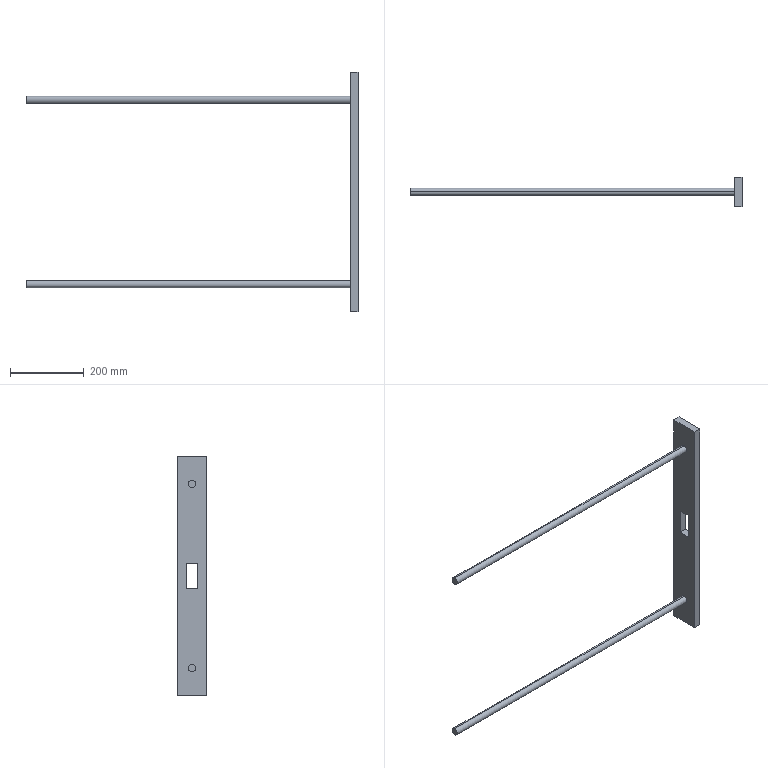Part | SolidWorks | features ICE 2, Extrusion 1 | 1 solid | 16 faces | box 900 x 80 x 650 mm | volume 1550920 mm3 | plane 12 | cylinder 4 | commonest cylinder face diameters 20 x4
STEP:
#1=CARTESIAN_POINT('',(-880.,0.,240.));
#2=VERTEX_POINT('',#1);
#3=CARTESIAN_POINT('',(-880.,0.,260.));
#4=VERTEX_POINT('',#3);
#5=CARTESIAN_POINT('',(-880.,0.,250.));
#6=DIRECTION('',(1.,0.,0.));
#7=DIRECTION('',(0.,0.,-1.));
#8=AXIS2_PLACEMENT_3D('',#5,#6,#7);
#9=CIRCLE('',#8,10.);
#10=EDGE_CURVE('',#2,#4,#9,.T.);
#11=ORIENTED_EDGE('',*,*,#10,.T.);
#12=CARTESIAN_POINT('',(0.,0.,260.));
#13=VERTEX_POINT('',#12);
#14=CARTESIAN_POINT('',(-880.,0.,260.));
#15=DIRECTION('',(1.,0.,0.));
#16=VECTOR('',#15,1000.);
#17=LINE('',#14,#16);
#18=EDGE_CURVE('',#4,#13,#17,.T.);
#19=ORIENTED_EDGE('',*,*,#18,.T.);
#20=CARTESIAN_POINT('',(0.,0.,240.));
#21=VERTEX_POINT('',#20);
#22=CARTESIAN_POINT('',(0.,0.,250.));
#23=DIRECTION('',(1.,0.,0.));
#24=DIRECTION('',(0.,0.,-1.));
#25=AXIS2_PLACEMENT_3D('',#22,#23,#24);
#26=CIRCLE('',#25,10.);
#27=EDGE_CURVE('',#21,#13,#26,.T.);
#28=ORIENTED_EDGE('',*,*,#27,.F.);
#29=CARTESIAN_POINT('',(-880.,0.,240.));
#30=DIRECTION('',(1.,0.,0.));
#31=VECTOR('',#30,1000.);
#32=LINE('',#29,#31);
#33=EDGE_CURVE('',#2,#21,#32,.T.);
#34=ORIENTED_EDGE('',*,*,#33,.F.);
#35=EDGE_LOOP('',(#11,#19,#28,#34));
#36=FACE_OUTER_BOUND('',#35,.T.);
#37=CARTESIAN_POINT('',(-880.,0.,250.));
#38=DIRECTION('',(1.,0.,0.));
#39=DIRECTION('',(0.,0.,-1.));
#40=AXIS2_PLACEMENT_3D('',#37,#38,#39);
#41=CYLINDRICAL_SURFACE('',#40,10.);
#42=ADVANCED_FACE('',(#36),#41,.T.);
#43=CARTESIAN_POINT('',(-880.,0.,-260.));
#44=VERTEX_POINT('',#43);
#45=CARTESIAN_POINT('',(-880.,0.,-240.));
#46=VERTEX_POINT('',#45);
#47=CARTESIAN_POINT('',(-880.,0.,-250.));
#48=DIRECTION('',(1.,0.,0.));
#49=DIRECTION('',(0.,0.,-1.));
#50=AXIS2_PLACEMENT_3D('',#47,#48,#49);
#51=CIRCLE('',#50,10.);
#52=EDGE_CURVE('',#44,#46,#51,.T.);
#53=ORIENTED_EDGE('',*,*,#52,.T.);
#54=CARTESIAN_POINT('',(0.,0.,-240.));
#55=VERTEX_POINT('',#54);
#56=CARTESIAN_POINT('',(-880.,0.,-240.));
#57=DIRECTION('',(1.,0.,0.));
#58=VECTOR('',#57,1000.);
#59=LINE('',#56,#58);
#60=EDGE_CURVE('',#46,#55,#59,.T.);
#61=ORIENTED_EDGE('',*,*,#60,.T.);
#62=CARTESIAN_POINT('',(0.,0.,-260.));
#63=VERTEX_POINT('',#62);
#64=CARTESIAN_POINT('',(0.,0.,-250.));
#65=DIRECTION('',(1.,0.,0.));
#66=DIRECTION('',(0.,0.,-1.));
#67=AXIS2_PLACEMENT_3D('',#64,#65,#66);
#68=CIRCLE('',#67,10.);
#69=EDGE_CURVE('',#63,#55,#68,.T.);
#70=ORIENTED_EDGE('',*,*,#69,.F.);
#71=CARTESIAN_POINT('',(-880.,0.,-260.));
#72=DIRECTION('',(1.,0.,0.));
#73=VECTOR('',#72,1000.);
#74=LINE('',#71,#73);
#75=EDGE_CURVE('',#44,#63,#74,.T.);
#76=ORIENTED_EDGE('',*,*,#75,.F.);
#77=EDGE_LOOP('',(#53,#61,#70,#76));
#78=FACE_OUTER_BOUND('',#77,.T.);
#79=CARTESIAN_POINT('',(-880.,0.,-250.));
#80=DIRECTION('',(1.,0.,0.));
#81=DIRECTION('',(0.,0.,-1.));
#82=AXIS2_PLACEMENT_3D('',#79,#80,#81);
#83=CYLINDRICAL_SURFACE('',#82,10.);
#84=ADVANCED_FACE('',(#78),#83,.T.);
#85=CARTESIAN_POINT('',(20.,15.,-35.));
#86=VERTEX_POINT('',#85);
#87=CARTESIAN_POINT('',(20.,15.,35.));
#88=VERTEX_POINT('',#87);
#89=CARTESIAN_POINT('',(20.,15.,35.));
#90=DIRECTION('',(0.,0.,1.));
#91=VECTOR('',#90,1000.);
#92=LINE('',#89,#91);
#93=EDGE_CURVE('',#86,#88,#92,.T.);
#94=ORIENTED_EDGE('',*,*,#93,.F.);
#95=CARTESIAN_POINT('',(20.,-15.,-35.));
#96=VERTEX_POINT('',#95);
#97=CARTESIAN_POINT('',(20.,15.,-35.));
#98=DIRECTION('',(0.,1.,0.));
#99=VECTOR('',#98,1000.);
#100=LINE('',#97,#99);
#101=EDGE_CURVE('',#96,#86,#100,.T.);
#102=ORIENTED_EDGE('',*,*,#101,.F.);
#103=CARTESIAN_POINT('',(20.,-15.,35.));
#104=VERTEX_POINT('',#103);
#105=CARTESIAN_POINT('',(20.,-15.,35.));
#106=DIRECTION('',(0.,0.,-1.));
#107=VECTOR('',#106,1000.);
#108=LINE('',#105,#107);
#109=EDGE_CURVE('',#104,#96,#108,.T.);
#110=ORIENTED_EDGE('',*,*,#109,.F.);
#111=CARTESIAN_POINT('',(20.,15.,35.));
#112=DIRECTION('',(0.,-1.,0.));
#113=VECTOR('',#112,1000.);
#114=LINE('',#111,#113);
#115=EDGE_CURVE('',#88,#104,#114,.T.);
#116=ORIENTED_EDGE('',*,*,#115,.F.);
#117=EDGE_LOOP('',(#94,#102,#110,#116));
#118=FACE_BOUND('',#117,.T.);
#119=CARTESIAN_POINT('',(20.,-40.,325.));
#120=VERTEX_POINT('',#119);
#121=CARTESIAN_POINT('',(20.,-40.,-325.));
#122=VERTEX_POINT('',#121);
#123=CARTESIAN_POINT('',(20.,-40.,325.));
#124=DIRECTION('',(0.,0.,-1.));
#125=VECTOR('',#124,1000.);
#126=LINE('',#123,#125);
#127=EDGE_CURVE('',#120,#122,#126,.T.);
#128=ORIENTED_EDGE('',*,*,#127,.T.);
#129=CARTESIAN_POINT('',(20.,40.,-325.));
#130=VERTEX_POINT('',#129);
#131=CARTESIAN_POINT('',(20.,-40.,-325.));
#132=DIRECTION('',(0.,1.,0.));
#133=VECTOR('',#132,1000.);
#134=LINE('',#131,#133);
#135=EDGE_CURVE('',#122,#130,#134,.T.);
#136=ORIENTED_EDGE('',*,*,#135,.T.);
#137=CARTESIAN_POINT('',(20.,40.,325.));
#138=VERTEX_POINT('',#137);
#139=CARTESIAN_POINT('',(20.,40.,325.));
#140=DIRECTION('',(0.,0.,1.));
#141=VECTOR('',#140,1000.);
#142=LINE('',#139,#141);
#143=EDGE_CURVE('',#130,#138,#142,.T.);
#144=ORIENTED_EDGE('',*,*,#143,.T.);
#145=CARTESIAN_POINT('',(20.,-40.,325.));
#146=DIRECTION('',(0.,-1.,0.));
#147=VECTOR('',#146,1000.);
#148=LINE('',#145,#147);
#149=EDGE_CURVE('',#138,#120,#148,.T.);
#150=ORIENTED_EDGE('',*,*,#149,.T.);
#151=EDGE_LOOP('',(#128,#136,#144,#150));
#152=FACE_OUTER_BOUND('',#151,.T.);
#153=CARTESIAN_POINT('',(20.,0.,0.));
#154=DIRECTION('',(1.,0.,0.));
#155=DIRECTION('',(0.,0.,-1.));
#156=AXIS2_PLACEMENT_3D('',#153,#154,#155);
#157=PLANE('',#156);
#158=ADVANCED_FACE('',(#118,#152),#157,.T.);
#159=CARTESIAN_POINT('',(0.,-15.,-35.));
#160=VERTEX_POINT('',#159);
#161=CARTESIAN_POINT('',(0.,15.,-35.));
#162=VERTEX_POINT('',#161);
#163=CARTESIAN_POINT('',(0.,15.,-35.));
#164=DIRECTION('',(0.,1.,0.));
#165=VECTOR('',#164,1000.);
#166=LINE('',#163,#165);
#167=EDGE_CURVE('',#160,#162,#166,.T.);
#168=ORIENTED_EDGE('',*,*,#167,.T.);
#169=CARTESIAN_POINT('',(0.,15.,35.));
#170=VERTEX_POINT('',#169);
#171=CARTESIAN_POINT('',(0.,15.,35.));
#172=DIRECTION('',(0.,0.,1.));
#173=VECTOR('',#172,1000.);
#174=LINE('',#171,#173);
#175=EDGE_CURVE('',#162,#170,#174,.T.);
#176=ORIENTED_EDGE('',*,*,#175,.T.);
#177=CARTESIAN_POINT('',(0.,-15.,35.));
#178=VERTEX_POINT('',#177);
#179=CARTESIAN_POINT('',(0.,15.,35.));
#180=DIRECTION('',(0.,-1.,0.));
#181=VECTOR('',#180,1000.);
#182=LINE('',#179,#181);
#183=EDGE_CURVE('',#170,#178,#182,.T.);
#184=ORIENTED_EDGE('',*,*,#183,.T.);
#185=CARTESIAN_POINT('',(0.,-15.,35.));
#186=DIRECTION('',(0.,0.,-1.));
#187=VECTOR('',#186,1000.);
#188=LINE('',#185,#187);
#189=EDGE_CURVE('',#178,#160,#188,.T.);
#190=ORIENTED_EDGE('',*,*,#189,.T.);
#191=EDGE_LOOP('',(#168,#176,#184,#190));
#192=FACE_BOUND('',#191,.T.);
#193=ORIENTED_EDGE('',*,*,#27,.T.);
#194=CARTESIAN_POINT('',(0.,0.,250.));
#195=DIRECTION('',(1.,0.,0.));
#196=DIRECTION('',(0.,0.,-1.));
#197=AXIS2_PLACEMENT_3D('',#194,#195,#196);
#198=CIRCLE('',#197,10.);
#199=EDGE_CURVE('',#13,#21,#198,.T.);
#200=ORIENTED_EDGE('',*,*,#199,.T.);
#201=EDGE_LOOP('',(#193,#200));
#202=FACE_BOUND('',#201,.T.);
#203=ORIENTED_EDGE('',*,*,#69,.T.);
#204=CARTESIAN_POINT('',(0.,0.,-250.));
#205=DIRECTION('',(1.,0.,0.));
#206=DIRECTION('',(0.,0.,-1.));
#207=AXIS2_PLACEMENT_3D('',#204,#205,#206);
#208=CIRCLE('',#207,10.);
#209=EDGE_CURVE('',#55,#63,#208,.T.);
#210=ORIENTED_EDGE('',*,*,#209,.T.);
#211=EDGE_LOOP('',(#203,#210));
#212=FACE_BOUND('',#211,.T.);
#213=CARTESIAN_POINT('',(0.,-40.,-325.));
#214=VERTEX_POINT('',#213);
#215=CARTESIAN_POINT('',(0.,40.,-325.));
#216=VERTEX_POINT('',#215);
#217=CARTESIAN_POINT('',(0.,0.,-325.));
#218=DIRECTION('',(0.,1.,0.));
#219=VECTOR('',#218,1000.);
#220=LINE('',#217,#219);
#221=EDGE_CURVE('',#214,#216,#220,.T.);
#222=ORIENTED_EDGE('',*,*,#221,.F.);
#223=CARTESIAN_POINT('',(0.,-40.,325.));
#224=VERTEX_POINT('',#223);
#225=CARTESIAN_POINT('',(0.,-40.,0.));
#226=DIRECTION('',(0.,0.,-1.));
#227=VECTOR('',#226,1000.);
#228=LINE('',#225,#227);
#229=EDGE_CURVE('',#224,#214,#228,.T.);
#230=ORIENTED_EDGE('',*,*,#229,.F.);
#231=CARTESIAN_POINT('',(0.,40.,325.));
#232=VERTEX_POINT('',#231);
#233=CARTESIAN_POINT('',(0.,0.,325.));
#234=DIRECTION('',(0.,-1.,0.));
#235=VECTOR('',#234,1000.);
#236=LINE('',#233,#235);
#237=EDGE_CURVE('',#232,#224,#236,.T.);
#238=ORIENTED_EDGE('',*,*,#237,.F.);
#239=CARTESIAN_POINT('',(0.,40.,0.));
#240=DIRECTION('',(0.,0.,1.));
#241=VECTOR('',#240,1000.);
#242=LINE('',#239,#241);
#243=EDGE_CURVE('',#216,#232,#242,.T.);
#244=ORIENTED_EDGE('',*,*,#243,.F.);
#245=EDGE_LOOP('',(#222,#230,#238,#244));
#246=FACE_OUTER_BOUND('',#245,.T.);
#247=CARTESIAN_POINT('',(0.,0.,0.));
#248=DIRECTION('',(1.,0.,0.));
#249=DIRECTION('',(0.,0.,-1.));
#250=AXIS2_PLACEMENT_3D('',#247,#248,#249);
#251=PLANE('',#250);
#252=ADVANCED_FACE('',(#192,#202,#212,#246),#251,.F.);
#253=ORIENTED_EDGE('',*,*,#167,.F.);
#254=CARTESIAN_POINT('',(20.,-15.,-35.));
#255=DIRECTION('',(-1.,0.,0.));
#256=VECTOR('',#255,1000.);
#257=LINE('',#254,#256);
#258=EDGE_CURVE('',#96,#160,#257,.T.);
#259=ORIENTED_EDGE('',*,*,#258,.F.);
#260=ORIENTED_EDGE('',*,*,#101,.T.);
#261=CARTESIAN_POINT('',(20.,15.,-35.));
#262=DIRECTION('',(-1.,0.,0.));
#263=VECTOR('',#262,1000.);
#264=LINE('',#261,#263);
#265=EDGE_CURVE('',#86,#162,#264,.T.);
#266=ORIENTED_EDGE('',*,*,#265,.T.);
#267=EDGE_LOOP('',(#253,#259,#260,#266));
#268=FACE_OUTER_BOUND('',#267,.T.);
#269=CARTESIAN_POINT('',(20.,15.,-35.));
#270=DIRECTION('',(0.,0.,1.));
#271=DIRECTION('',(0.,-1.,0.));
#272=AXIS2_PLACEMENT_3D('',#269,#270,#271);
#273=PLANE('',#272);
#274=ADVANCED_FACE('',(#268),#273,.T.);
#275=ORIENTED_EDGE('',*,*,#175,.F.);
#276=ORIENTED_EDGE('',*,*,#265,.F.);
#277=ORIENTED_EDGE('',*,*,#93,.T.);
#278=CARTESIAN_POINT('',(20.,15.,35.));
#279=DIRECTION('',(-1.,0.,0.));
#280=VECTOR('',#279,1000.);
#281=LINE('',#278,#280);
#282=EDGE_CURVE('',#88,#170,#281,.T.);
#283=ORIENTED_EDGE('',*,*,#282,.T.);
#284=EDGE_LOOP('',(#275,#276,#277,#283));
#285=FACE_OUTER_BOUND('',#284,.T.);
#286=CARTESIAN_POINT('',(20.,15.,35.));
#287=DIRECTION('',(0.,-1.,0.));
#288=DIRECTION('',(0.,0.,-1.));
#289=AXIS2_PLACEMENT_3D('',#286,#287,#288);
#290=PLANE('',#289);
#291=ADVANCED_FACE('',(#285),#290,.T.);
#292=ORIENTED_EDGE('',*,*,#183,.F.);
#293=ORIENTED_EDGE('',*,*,#282,.F.);
#294=ORIENTED_EDGE('',*,*,#115,.T.);
#295=CARTESIAN_POINT('',(20.,-15.,35.));
#296=DIRECTION('',(-1.,0.,0.));
#297=VECTOR('',#296,1000.);
#298=LINE('',#295,#297);
#299=EDGE_CURVE('',#104,#178,#298,.T.);
#300=ORIENTED_EDGE('',*,*,#299,.T.);
#301=EDGE_LOOP('',(#292,#293,#294,#300));
#302=FACE_OUTER_BOUND('',#301,.T.);
#303=CARTESIAN_POINT('',(20.,15.,35.));
#304=DIRECTION('',(0.,0.,-1.));
#305=DIRECTION('',(0.,1.,0.));
#306=AXIS2_PLACEMENT_3D('',#303,#304,#305);
#307=PLANE('',#306);
#308=ADVANCED_FACE('',(#302),#307,.T.);
#309=ORIENTED_EDGE('',*,*,#189,.F.);
#310=ORIENTED_EDGE('',*,*,#299,.F.);
#311=ORIENTED_EDGE('',*,*,#109,.T.);
#312=ORIENTED_EDGE('',*,*,#258,.T.);
#313=EDGE_LOOP('',(#309,#310,#311,#312));
#314=FACE_OUTER_BOUND('',#313,.T.);
#315=CARTESIAN_POINT('',(20.,-15.,35.));
#316=DIRECTION('',(0.,1.,0.));
#317=DIRECTION('',(0.,0.,1.));
#318=AXIS2_PLACEMENT_3D('',#315,#316,#317);
#319=PLANE('',#318);
#320=ADVANCED_FACE('',(#314),#319,.T.);
#321=ORIENTED_EDGE('',*,*,#60,.F.);
#322=CARTESIAN_POINT('',(-880.,0.,-250.));
#323=DIRECTION('',(1.,0.,0.));
#324=DIRECTION('',(0.,0.,-1.));
#325=AXIS2_PLACEMENT_3D('',#322,#323,#324);
#326=CIRCLE('',#325,10.);
#327=EDGE_CURVE('',#46,#44,#326,.T.);
#328=ORIENTED_EDGE('',*,*,#327,.T.);
#329=ORIENTED_EDGE('',*,*,#75,.T.);
#330=ORIENTED_EDGE('',*,*,#209,.F.);
#331=EDGE_LOOP('',(#321,#328,#329,#330));
#332=FACE_OUTER_BOUND('',#331,.T.);
#333=CARTESIAN_POINT('',(-880.,0.,-250.));
#334=DIRECTION('',(1.,0.,0.));
#335=DIRECTION('',(0.,0.,-1.));
#336=AXIS2_PLACEMENT_3D('',#333,#334,#335);
#337=CYLINDRICAL_SURFACE('',#336,10.);
#338=ADVANCED_FACE('',(#332),#337,.T.);
#339=ORIENTED_EDGE('',*,*,#52,.F.);
#340=ORIENTED_EDGE('',*,*,#327,.F.);
#341=EDGE_LOOP('',(#339,#340));
#342=FACE_OUTER_BOUND('',#341,.T.);
#343=CARTESIAN_POINT('',(-880.,0.,-250.));
#344=DIRECTION('',(1.,0.,0.));
#345=DIRECTION('',(0.,0.,-1.));
#346=AXIS2_PLACEMENT_3D('',#343,#344,#345);
#347=PLANE('',#346);
#348=ADVANCED_FACE('',(#342),#347,.F.);
#349=ORIENTED_EDGE('',*,*,#18,.F.);
#350=CARTESIAN_POINT('',(-880.,0.,250.));
#351=DIRECTION('',(1.,0.,0.));
#352=DIRECTION('',(0.,0.,-1.));
#353=AXIS2_PLACEMENT_3D('',#350,#351,#352);
#354=CIRCLE('',#353,10.);
#355=EDGE_CURVE('',#4,#2,#354,.T.);
#356=ORIENTED_EDGE('',*,*,#355,.T.);
#357=ORIENTED_EDGE('',*,*,#33,.T.);
#358=ORIENTED_EDGE('',*,*,#199,.F.);
#359=EDGE_LOOP('',(#349,#356,#357,#358));
#360=FACE_OUTER_BOUND('',#359,.T.);
#361=CARTESIAN_POINT('',(-880.,0.,250.));
#362=DIRECTION('',(1.,0.,0.));
#363=DIRECTION('',(0.,0.,-1.));
#364=AXIS2_PLACEMENT_3D('',#361,#362,#363);
#365=CYLINDRICAL_SURFACE('',#364,10.);
#366=ADVANCED_FACE('',(#360),#365,.T.);
#367=ORIENTED_EDGE('',*,*,#10,.F.);
#368=ORIENTED_EDGE('',*,*,#355,.F.);
#369=EDGE_LOOP('',(#367,#368));
#370=FACE_OUTER_BOUND('',#369,.T.);
#371=CARTESIAN_POINT('',(-880.,0.,250.));
#372=DIRECTION('',(1.,0.,0.));
#373=DIRECTION('',(0.,0.,-1.));
#374=AXIS2_PLACEMENT_3D('',#371,#372,#373);
#375=PLANE('',#374);
#376=ADVANCED_FACE('',(#370),#375,.F.);
#377=ORIENTED_EDGE('',*,*,#221,.T.);
#378=CARTESIAN_POINT('',(-880.,40.,-325.));
#379=DIRECTION('',(1.,0.,0.));
#380=VECTOR('',#379,1000.);
#381=LINE('',#378,#380);
#382=EDGE_CURVE('',#216,#130,#381,.T.);
#383=ORIENTED_EDGE('',*,*,#382,.T.);
#384=ORIENTED_EDGE('',*,*,#135,.F.);
#385=CARTESIAN_POINT('',(-880.,-40.,-325.));
#386=DIRECTION('',(1.,0.,0.));
#387=VECTOR('',#386,1000.);
#388=LINE('',#385,#387);
#389=EDGE_CURVE('',#214,#122,#388,.T.);
#390=ORIENTED_EDGE('',*,*,#389,.F.);
#391=EDGE_LOOP('',(#377,#383,#384,#390));
#392=FACE_OUTER_BOUND('',#391,.T.);
#393=CARTESIAN_POINT('',(-880.,-40.,-325.));
#394=DIRECTION('',(0.,0.,-1.));
#395=DIRECTION('',(-1.,0.,0.));
#396=AXIS2_PLACEMENT_3D('',#393,#394,#395);
#397=PLANE('',#396);
#398=ADVANCED_FACE('',(#392),#397,.T.);
#399=ORIENTED_EDGE('',*,*,#229,.T.);
#400=ORIENTED_EDGE('',*,*,#389,.T.);
#401=ORIENTED_EDGE('',*,*,#127,.F.);
#402=CARTESIAN_POINT('',(-880.,-40.,325.));
#403=DIRECTION('',(1.,0.,0.));
#404=VECTOR('',#403,1000.);
#405=LINE('',#402,#404);
#406=EDGE_CURVE('',#224,#120,#405,.T.);
#407=ORIENTED_EDGE('',*,*,#406,.F.);
#408=EDGE_LOOP('',(#399,#400,#401,#407));
#409=FACE_OUTER_BOUND('',#408,.T.);
#410=CARTESIAN_POINT('',(-880.,-40.,325.));
#411=DIRECTION('',(0.,-1.,0.));
#412=DIRECTION('',(0.,0.,-1.));
#413=AXIS2_PLACEMENT_3D('',#410,#411,#412);
#414=PLANE('',#413);
#415=ADVANCED_FACE('',(#409),#414,.T.);
#416=ORIENTED_EDGE('',*,*,#237,.T.);
#417=ORIENTED_EDGE('',*,*,#406,.T.);
#418=ORIENTED_EDGE('',*,*,#149,.F.);
#419=CARTESIAN_POINT('',(-880.,40.,325.));
#420=DIRECTION('',(1.,0.,0.));
#421=VECTOR('',#420,1000.);
#422=LINE('',#419,#421);
#423=EDGE_CURVE('',#232,#138,#422,.T.);
#424=ORIENTED_EDGE('',*,*,#423,.F.);
#425=EDGE_LOOP('',(#416,#417,#418,#424));
#426=FACE_OUTER_BOUND('',#425,.T.);
#427=CARTESIAN_POINT('',(-880.,-40.,325.));
#428=DIRECTION('',(0.,0.,1.));
#429=DIRECTION('',(1.,0.,0.));
#430=AXIS2_PLACEMENT_3D('',#427,#428,#429);
#431=PLANE('',#430);
#432=ADVANCED_FACE('',(#426),#431,.T.);
#433=ORIENTED_EDGE('',*,*,#243,.T.);
#434=ORIENTED_EDGE('',*,*,#423,.T.);
#435=ORIENTED_EDGE('',*,*,#143,.F.);
#436=ORIENTED_EDGE('',*,*,#382,.F.);
#437=EDGE_LOOP('',(#433,#434,#435,#436));
#438=FACE_OUTER_BOUND('',#437,.T.);
#439=CARTESIAN_POINT('',(-880.,40.,325.));
#440=DIRECTION('',(0.,1.,0.));
#441=DIRECTION('',(0.,0.,1.));
#442=AXIS2_PLACEMENT_3D('',#439,#440,#441);
#443=PLANE('',#442);
#444=ADVANCED_FACE('',(#438),#443,.T.);
#445=CLOSED_SHELL('',(#42,#84,#158,#252,#274,#291,#308,#320,#338,#348,#366,#376,#398,#415,#432,#444));
#446=MANIFOLD_SOLID_BREP('',#445);
#447=CARTESIAN_POINT('',(0.,0.,0.));
#448=DIRECTION('',(0.,0.,1.));
#449=DIRECTION('',(1.,0.,0.));
#450=AXIS2_PLACEMENT_3D('',#447,#448,#449);
#451=(LENGTH_UNIT()NAMED_UNIT(*)SI_UNIT(.MILLI.,.METRE.));
#452=UNCERTAINTY_MEASURE_WITH_UNIT(LENGTH_MEASURE(0.00001),#451,'','');
#453=(NAMED_UNIT(*)PLANE_ANGLE_UNIT()SI_UNIT($,.RADIAN.));
#454=(NAMED_UNIT(*)SI_UNIT($,.STERADIAN.)SOLID_ANGLE_UNIT());
#455=(GEOMETRIC_REPRESENTATION_CONTEXT(3)GLOBAL_UNCERTAINTY_ASSIGNED_CONTEXT((#452))GLOBAL_UNIT_ASSIGNED_CONTEXT((#451,#453,#454))REPRESENTATION_CONTEXT('',''));
#456=ADVANCED_BREP_SHAPE_REPRESENTATION('',(#446,#450),#455);